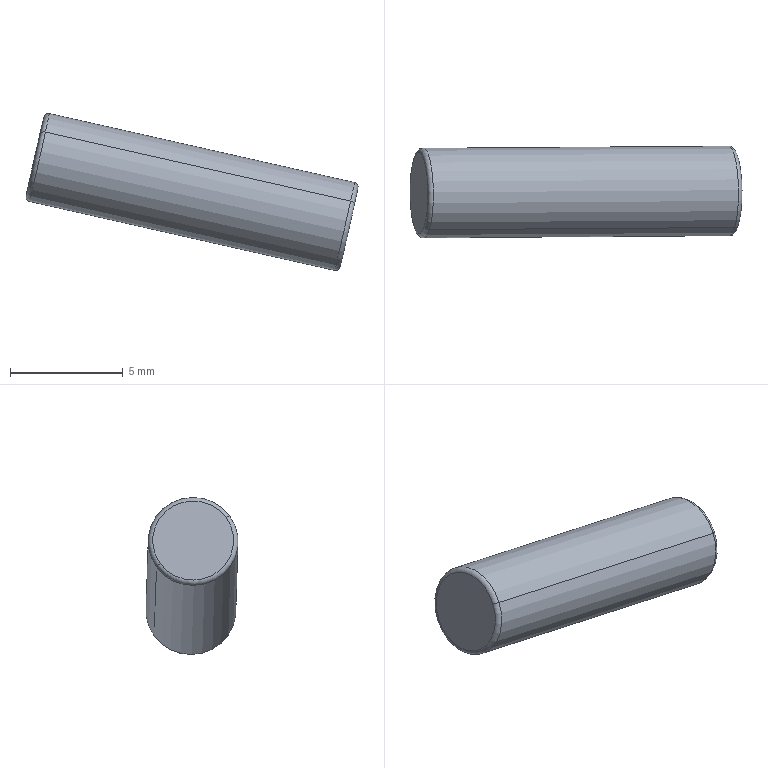Part | SolidWorks | features BaseBody 1 | 1 solid | 8 faces | box 14.752 x 4.1 x 6.976 mm | volume 179.488 mm3 | torus 4 | cylinder 2 | plane 2 | commonest cylinder face diameters 4 x2
STEP:
#1=CARTESIAN_POINT('',(1961.793,-247.623,1004.545));
#2=VERTEX_POINT('',#1);
#3=CARTESIAN_POINT('',(1961.961,-247.459,1004.388));
#4=VERTEX_POINT('',#3);
#5=CARTESIAN_POINT('',(1961.988,-247.621,1004.501));
#6=DIRECTION('',(-0.1754,-0.5807,-0.795));
#7=DIRECTION('',(0.1337,-0.8141,0.5651));
#8=AXIS2_PLACEMENT_3D('',#5,#6,#7);
#9=CIRCLE('',#8,0.2);
#10=EDGE_CURVE('',#2,#4,#9,.T.);
#11=ORIENTED_EDGE('',*,*,#10,.T.);
#12=CARTESIAN_POINT('',(1962.496,-250.715,1006.649));
#13=VERTEX_POINT('',#12);
#14=CARTESIAN_POINT('',(1962.228,-249.087,1005.519));
#15=DIRECTION('',(0.9754,0.007201,-0.2205));
#16=DIRECTION('',(-0.08981,-0.8999,-0.4268));
#17=AXIS2_PLACEMENT_3D('',#14,#15,#16);
#18=CIRCLE('',#17,2.);
#19=EDGE_CURVE('',#13,#4,#18,.T.);
#20=ORIENTED_EDGE('',*,*,#19,.F.);
#21=CARTESIAN_POINT('',(1962.274,-250.554,1006.58));
#22=VERTEX_POINT('',#21);
#23=CARTESIAN_POINT('',(1962.469,-250.552,1006.536));
#24=DIRECTION('',(-0.1754,-0.5807,-0.795));
#25=DIRECTION('',(0.1337,-0.8141,0.5651));
#26=AXIS2_PLACEMENT_3D('',#23,#24,#25);
#27=CIRCLE('',#26,0.2);
#28=EDGE_CURVE('',#13,#22,#27,.T.);
#29=ORIENTED_EDGE('',*,*,#28,.T.);
#30=CARTESIAN_POINT('',(1962.033,-249.088,1005.563));
#31=DIRECTION('',(0.9754,0.007201,-0.2205));
#32=DIRECTION('',(-0.08981,-0.8999,-0.4268));
#33=AXIS2_PLACEMENT_3D('',#30,#31,#32);
#34=CIRCLE('',#33,1.8);
#35=EDGE_CURVE('',#22,#2,#34,.T.);
#36=ORIENTED_EDGE('',*,*,#35,.T.);
#37=EDGE_LOOP('',(#11,#20,#29,#36));
#38=FACE_OUTER_BOUND('',#37,.T.);
#39=CARTESIAN_POINT('',(1962.228,-249.087,1005.519));
#40=DIRECTION('',(0.9754,0.007201,-0.2205));
#41=DIRECTION('',(-0.1337,0.8141,-0.5651));
#42=AXIS2_PLACEMENT_3D('',#39,#40,#41);
#43=TOROIDAL_SURFACE('',#42,1.8,0.2);
#44=ADVANCED_FACE('',(#38),#43,.T.);
#45=ORIENTED_EDGE('',*,*,#28,.F.);
#46=CARTESIAN_POINT('',(1962.228,-249.087,1005.519));
#47=DIRECTION('',(0.9754,0.007201,-0.2205));
#48=DIRECTION('',(-0.08981,-0.8999,-0.4268));
#49=AXIS2_PLACEMENT_3D('',#46,#47,#48);
#50=CIRCLE('',#49,2.);
#51=EDGE_CURVE('',#4,#13,#50,.T.);
#52=ORIENTED_EDGE('',*,*,#51,.F.);
#53=ORIENTED_EDGE('',*,*,#10,.F.);
#54=CARTESIAN_POINT('',(1962.033,-249.088,1005.563));
#55=DIRECTION('',(0.9754,0.007201,-0.2205));
#56=DIRECTION('',(-0.08981,-0.8999,-0.4268));
#57=AXIS2_PLACEMENT_3D('',#54,#55,#56);
#58=CIRCLE('',#57,1.8);
#59=EDGE_CURVE('',#2,#22,#58,.T.);
#60=ORIENTED_EDGE('',*,*,#59,.T.);
#61=EDGE_LOOP('',(#45,#52,#53,#60));
#62=FACE_OUTER_BOUND('',#61,.T.);
#63=CARTESIAN_POINT('',(1962.228,-249.087,1005.519));
#64=DIRECTION('',(0.9754,0.007201,-0.2205));
#65=DIRECTION('',(-0.1337,0.8141,-0.5651));
#66=AXIS2_PLACEMENT_3D('',#63,#64,#65);
#67=TOROIDAL_SURFACE('',#66,1.8,0.2);
#68=ADVANCED_FACE('',(#62),#67,.T.);
#69=CARTESIAN_POINT('',(1975.519,-247.359,1001.324));
#70=VERTEX_POINT('',#69);
#71=CARTESIAN_POINT('',(1968.74,-247.409,1002.856));
#72=DIRECTION('',(0.9754,0.007201,-0.2205));
#73=VECTOR('',#72,1000.);
#74=LINE('',#71,#73);
#75=EDGE_CURVE('',#4,#70,#74,.T.);
#76=ORIENTED_EDGE('',*,*,#75,.T.);
#77=CARTESIAN_POINT('',(1976.054,-250.615,1003.584));
#78=VERTEX_POINT('',#77);
#79=CARTESIAN_POINT('',(1975.786,-248.987,1002.454));
#80=DIRECTION('',(0.9754,0.007201,-0.2205));
#81=DIRECTION('',(-0.08981,-0.8999,-0.4268));
#82=AXIS2_PLACEMENT_3D('',#79,#80,#81);
#83=CIRCLE('',#82,2.);
#84=EDGE_CURVE('',#78,#70,#83,.T.);
#85=ORIENTED_EDGE('',*,*,#84,.F.);
#86=CARTESIAN_POINT('',(1969.275,-250.665,1005.117));
#87=DIRECTION('',(-0.9754,-0.007201,0.2205));
#88=VECTOR('',#87,1000.);
#89=LINE('',#86,#88);
#90=EDGE_CURVE('',#78,#13,#89,.T.);
#91=ORIENTED_EDGE('',*,*,#90,.T.);
#92=ORIENTED_EDGE('',*,*,#19,.T.);
#93=EDGE_LOOP('',(#76,#85,#91,#92));
#94=FACE_OUTER_BOUND('',#93,.T.);
#95=CARTESIAN_POINT('',(1969.007,-249.037,1003.986));
#96=DIRECTION('',(0.9754,0.007201,-0.2205));
#97=DIRECTION('',(-0.1337,0.8141,-0.5651));
#98=AXIS2_PLACEMENT_3D('',#95,#96,#97);
#99=CYLINDRICAL_SURFACE('',#98,2.);
#100=ADVANCED_FACE('',(#94),#99,.T.);
#101=ORIENTED_EDGE('',*,*,#90,.F.);
#102=CARTESIAN_POINT('',(1975.786,-248.987,1002.454));
#103=DIRECTION('',(0.9754,0.007201,-0.2205));
#104=DIRECTION('',(-0.08981,-0.8999,-0.4268));
#105=AXIS2_PLACEMENT_3D('',#102,#103,#104);
#106=CIRCLE('',#105,2.);
#107=EDGE_CURVE('',#70,#78,#106,.T.);
#108=ORIENTED_EDGE('',*,*,#107,.F.);
#109=ORIENTED_EDGE('',*,*,#75,.F.);
#110=ORIENTED_EDGE('',*,*,#51,.T.);
#111=EDGE_LOOP('',(#101,#108,#109,#110));
#112=FACE_OUTER_BOUND('',#111,.T.);
#113=CARTESIAN_POINT('',(1969.007,-249.037,1003.986));
#114=DIRECTION('',(0.9754,0.007201,-0.2205));
#115=DIRECTION('',(-0.1337,0.8141,-0.5651));
#116=AXIS2_PLACEMENT_3D('',#113,#114,#115);
#117=CYLINDRICAL_SURFACE('',#116,2.);
#118=ADVANCED_FACE('',(#112),#117,.T.);
#119=CARTESIAN_POINT('',(1975.74,-247.52,1001.393));
#120=VERTEX_POINT('',#119);
#121=CARTESIAN_POINT('',(1975.545,-247.521,1001.437));
#122=DIRECTION('',(-0.1754,-0.5807,-0.795));
#123=DIRECTION('',(0.1337,-0.8141,0.5651));
#124=AXIS2_PLACEMENT_3D('',#121,#122,#123);
#125=CIRCLE('',#124,0.2);
#126=EDGE_CURVE('',#70,#120,#125,.T.);
#127=ORIENTED_EDGE('',*,*,#126,.T.);
#128=CARTESIAN_POINT('',(1976.222,-250.451,1003.427));
#129=VERTEX_POINT('',#128);
#130=CARTESIAN_POINT('',(1975.981,-248.985,1002.41));
#131=DIRECTION('',(0.9754,0.007201,-0.2205));
#132=DIRECTION('',(-0.08981,-0.8999,-0.4268));
#133=AXIS2_PLACEMENT_3D('',#130,#131,#132);
#134=CIRCLE('',#133,1.8);
#135=EDGE_CURVE('',#129,#120,#134,.T.);
#136=ORIENTED_EDGE('',*,*,#135,.F.);
#137=CARTESIAN_POINT('',(1976.027,-250.452,1003.471));
#138=DIRECTION('',(-0.1754,-0.5807,-0.795));
#139=DIRECTION('',(0.1337,-0.8141,0.5651));
#140=AXIS2_PLACEMENT_3D('',#137,#138,#139);
#141=CIRCLE('',#140,0.2);
#142=EDGE_CURVE('',#129,#78,#141,.T.);
#143=ORIENTED_EDGE('',*,*,#142,.T.);
#144=ORIENTED_EDGE('',*,*,#84,.T.);
#145=EDGE_LOOP('',(#127,#136,#143,#144));
#146=FACE_OUTER_BOUND('',#145,.T.);
#147=CARTESIAN_POINT('',(1975.786,-248.987,1002.454));
#148=DIRECTION('',(0.9754,0.007201,-0.2205));
#149=DIRECTION('',(-0.1337,0.8141,-0.5651));
#150=AXIS2_PLACEMENT_3D('',#147,#148,#149);
#151=TOROIDAL_SURFACE('',#150,1.8,0.2);
#152=ADVANCED_FACE('',(#146),#151,.T.);
#153=ORIENTED_EDGE('',*,*,#142,.F.);
#154=CARTESIAN_POINT('',(1975.981,-248.985,1002.41));
#155=DIRECTION('',(0.9754,0.007201,-0.2205));
#156=DIRECTION('',(-0.08981,-0.8999,-0.4268));
#157=AXIS2_PLACEMENT_3D('',#154,#155,#156);
#158=CIRCLE('',#157,1.8);
#159=EDGE_CURVE('',#120,#129,#158,.T.);
#160=ORIENTED_EDGE('',*,*,#159,.F.);
#161=ORIENTED_EDGE('',*,*,#126,.F.);
#162=ORIENTED_EDGE('',*,*,#107,.T.);
#163=EDGE_LOOP('',(#153,#160,#161,#162));
#164=FACE_OUTER_BOUND('',#163,.T.);
#165=CARTESIAN_POINT('',(1975.786,-248.987,1002.454));
#166=DIRECTION('',(0.9754,0.007201,-0.2205));
#167=DIRECTION('',(-0.1337,0.8141,-0.5651));
#168=AXIS2_PLACEMENT_3D('',#165,#166,#167);
#169=TOROIDAL_SURFACE('',#168,1.8,0.2);
#170=ADVANCED_FACE('',(#164),#169,.T.);
#171=ORIENTED_EDGE('',*,*,#59,.F.);
#172=ORIENTED_EDGE('',*,*,#35,.F.);
#173=EDGE_LOOP('',(#171,#172));
#174=FACE_OUTER_BOUND('',#173,.T.);
#175=CARTESIAN_POINT('',(1962.396,-249.873,1007.141));
#176=DIRECTION('',(0.9754,0.007201,-0.2205));
#177=DIRECTION('',(0.08981,0.8999,0.4268));
#178=AXIS2_PLACEMENT_3D('',#175,#176,#177);
#179=PLANE('',#178);
#180=ADVANCED_FACE('',(#174),#179,.F.);
#181=ORIENTED_EDGE('',*,*,#159,.T.);
#182=ORIENTED_EDGE('',*,*,#135,.T.);
#183=EDGE_LOOP('',(#181,#182));
#184=FACE_OUTER_BOUND('',#183,.T.);
#185=CARTESIAN_POINT('',(1976.344,-249.77,1003.989));
#186=DIRECTION('',(0.9754,0.007201,-0.2205));
#187=DIRECTION('',(0.08981,0.8999,0.4268));
#188=AXIS2_PLACEMENT_3D('',#185,#186,#187);
#189=PLANE('',#188);
#190=ADVANCED_FACE('',(#184),#189,.T.);
#191=CLOSED_SHELL('',(#44,#68,#100,#118,#152,#170,#180,#190));
#192=MANIFOLD_SOLID_BREP('',#191);
#193=CARTESIAN_POINT('',(0.,0.,0.));
#194=DIRECTION('',(0.,0.,1.));
#195=DIRECTION('',(1.,0.,0.));
#196=AXIS2_PLACEMENT_3D('',#193,#194,#195);
#197=(LENGTH_UNIT()NAMED_UNIT(*)SI_UNIT(.MILLI.,.METRE.));
#198=UNCERTAINTY_MEASURE_WITH_UNIT(LENGTH_MEASURE(0.00001),#197,'','');
#199=(NAMED_UNIT(*)PLANE_ANGLE_UNIT()SI_UNIT($,.RADIAN.));
#200=(NAMED_UNIT(*)SI_UNIT($,.STERADIAN.)SOLID_ANGLE_UNIT());
#201=(GEOMETRIC_REPRESENTATION_CONTEXT(3)GLOBAL_UNCERTAINTY_ASSIGNED_CONTEXT((#198))GLOBAL_UNIT_ASSIGNED_CONTEXT((#197,#199,#200))REPRESENTATION_CONTEXT('',''));
#202=ADVANCED_BREP_SHAPE_REPRESENTATION('',(#192,#196),#201);